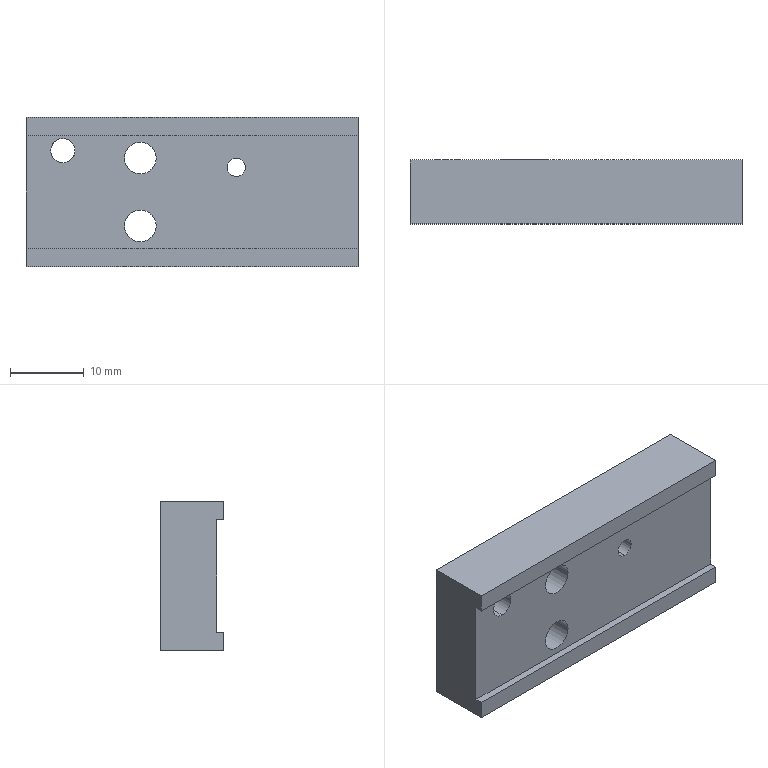Part | NX | 1 solid | 28 faces | box 45 x 8.65 x 20.2 mm | volume 6534 mm3 | plane 12 | cylinder 12 | cone 4 | commonest cylinder face diameters 4.3 x4 8 x4 2.5 x2 3.3 x2
STEP:
#1=CARTESIAN_POINT('',(45.,-1.,0.));
#2=VERTEX_POINT('',#1);
#3=CARTESIAN_POINT('',(45.,7.65,0.));
#4=VERTEX_POINT('',#3);
#5=CARTESIAN_POINT('',(45.,-1.,0.));
#6=DIRECTION('',(0.,1.,0.));
#7=VECTOR('',#6,1000.);
#8=LINE('',#5,#7);
#9=EDGE_CURVE('',#2,#4,#8,.T.);
#10=ORIENTED_EDGE('',*,*,#9,.T.);
#11=CARTESIAN_POINT('',(0.,7.65,0.));
#12=VERTEX_POINT('',#11);
#13=CARTESIAN_POINT('',(0.,7.65,0.));
#14=DIRECTION('',(-1.,0.,0.));
#15=VECTOR('',#14,1000.);
#16=LINE('',#13,#15);
#17=EDGE_CURVE('',#4,#12,#16,.T.);
#18=ORIENTED_EDGE('',*,*,#17,.T.);
#19=CARTESIAN_POINT('',(0.,-1.,0.));
#20=VERTEX_POINT('',#19);
#21=CARTESIAN_POINT('',(0.,7.65,0.));
#22=DIRECTION('',(0.,-1.,0.));
#23=VECTOR('',#22,1000.);
#24=LINE('',#21,#23);
#25=EDGE_CURVE('',#12,#20,#24,.T.);
#26=ORIENTED_EDGE('',*,*,#25,.T.);
#27=CARTESIAN_POINT('',(0.,-1.,0.));
#28=DIRECTION('',(1.,0.,0.));
#29=VECTOR('',#28,1000.);
#30=LINE('',#27,#29);
#31=EDGE_CURVE('',#20,#2,#30,.T.);
#32=ORIENTED_EDGE('',*,*,#31,.T.);
#33=EDGE_LOOP('',(#10,#18,#26,#32));
#34=FACE_BOUND('',#33,.T.);
#35=CARTESIAN_POINT('',(0.,0.,0.));
#36=DIRECTION('',(0.,0.,1.));
#37=DIRECTION('',(1.,0.,0.));
#38=AXIS2_PLACEMENT_3D('',#35,#36,#37);
#39=PLANE('',#38);
#40=ADVANCED_FACE('',(#34),#39,.T.);
#41=CARTESIAN_POINT('',(45.,7.65,-20.2));
#42=VERTEX_POINT('',#41);
#43=CARTESIAN_POINT('',(45.,-1.,-20.2));
#44=VERTEX_POINT('',#43);
#45=CARTESIAN_POINT('',(45.,7.65,-20.2));
#46=DIRECTION('',(0.,-1.,0.));
#47=VECTOR('',#46,1000.);
#48=LINE('',#45,#47);
#49=EDGE_CURVE('',#42,#44,#48,.T.);
#50=ORIENTED_EDGE('',*,*,#49,.F.);
#51=CARTESIAN_POINT('',(45.,7.65,0.));
#52=DIRECTION('',(0.,0.,1.));
#53=VECTOR('',#52,1000.);
#54=LINE('',#51,#53);
#55=EDGE_CURVE('',#42,#4,#54,.T.);
#56=ORIENTED_EDGE('',*,*,#55,.T.);
#57=ORIENTED_EDGE('',*,*,#9,.F.);
#58=CARTESIAN_POINT('',(45.,-1.,-2.5));
#59=VERTEX_POINT('',#58);
#60=CARTESIAN_POINT('',(45.,-1.,0.));
#61=DIRECTION('',(0.,0.,-1.));
#62=VECTOR('',#61,1000.);
#63=LINE('',#60,#62);
#64=EDGE_CURVE('',#2,#59,#63,.T.);
#65=ORIENTED_EDGE('',*,*,#64,.T.);
#66=CARTESIAN_POINT('',(45.,0.,-2.5));
#67=VERTEX_POINT('',#66);
#68=CARTESIAN_POINT('',(45.,-1.,-2.5));
#69=DIRECTION('',(0.,1.,0.));
#70=VECTOR('',#69,1000.);
#71=LINE('',#68,#70);
#72=EDGE_CURVE('',#59,#67,#71,.T.);
#73=ORIENTED_EDGE('',*,*,#72,.T.);
#74=CARTESIAN_POINT('',(45.,0.,-17.7));
#75=VERTEX_POINT('',#74);
#76=CARTESIAN_POINT('',(45.,0.,0.));
#77=DIRECTION('',(0.,0.,-1.));
#78=VECTOR('',#77,1000.);
#79=LINE('',#76,#78);
#80=EDGE_CURVE('',#67,#75,#79,.T.);
#81=ORIENTED_EDGE('',*,*,#80,.T.);
#82=CARTESIAN_POINT('',(45.,-1.,-17.7));
#83=VERTEX_POINT('',#82);
#84=CARTESIAN_POINT('',(45.,-1.,-17.7));
#85=DIRECTION('',(0.,1.,0.));
#86=VECTOR('',#85,1000.);
#87=LINE('',#84,#86);
#88=EDGE_CURVE('',#83,#75,#87,.T.);
#89=ORIENTED_EDGE('',*,*,#88,.F.);
#90=CARTESIAN_POINT('',(45.,-1.,-17.7));
#91=DIRECTION('',(0.,0.,-1.));
#92=VECTOR('',#91,1000.);
#93=LINE('',#90,#92);
#94=EDGE_CURVE('',#83,#44,#93,.T.);
#95=ORIENTED_EDGE('',*,*,#94,.T.);
#96=EDGE_LOOP('',(#50,#56,#57,#65,#73,#81,#89,#95));
#97=FACE_BOUND('',#96,.T.);
#98=CARTESIAN_POINT('',(45.,0.,0.));
#99=DIRECTION('',(1.,0.,0.));
#100=DIRECTION('',(0.,1.,0.));
#101=AXIS2_PLACEMENT_3D('',#98,#99,#100);
#102=PLANE('',#101);
#103=ADVANCED_FACE('',(#97),#102,.T.);
#104=CARTESIAN_POINT('',(0.,-1.,-20.2));
#105=VERTEX_POINT('',#104);
#106=CARTESIAN_POINT('',(0.,7.65,-20.2));
#107=VERTEX_POINT('',#106);
#108=CARTESIAN_POINT('',(0.,-1.,-20.2));
#109=DIRECTION('',(0.,1.,0.));
#110=VECTOR('',#109,1000.);
#111=LINE('',#108,#110);
#112=EDGE_CURVE('',#105,#107,#111,.T.);
#113=ORIENTED_EDGE('',*,*,#112,.T.);
#114=CARTESIAN_POINT('',(0.,7.65,-20.2));
#115=DIRECTION('',(-1.,0.,0.));
#116=VECTOR('',#115,1000.);
#117=LINE('',#114,#116);
#118=EDGE_CURVE('',#42,#107,#117,.T.);
#119=ORIENTED_EDGE('',*,*,#118,.F.);
#120=ORIENTED_EDGE('',*,*,#49,.T.);
#121=CARTESIAN_POINT('',(45.,-1.,-20.2));
#122=DIRECTION('',(-1.,0.,0.));
#123=VECTOR('',#122,1000.);
#124=LINE('',#121,#123);
#125=EDGE_CURVE('',#44,#105,#124,.T.);
#126=ORIENTED_EDGE('',*,*,#125,.T.);
#127=EDGE_LOOP('',(#113,#119,#120,#126));
#128=FACE_BOUND('',#127,.T.);
#129=CARTESIAN_POINT('',(0.,0.,-20.2));
#130=DIRECTION('',(0.,0.,1.));
#131=DIRECTION('',(1.,0.,0.));
#132=AXIS2_PLACEMENT_3D('',#129,#130,#131);
#133=PLANE('',#132);
#134=ADVANCED_FACE('',(#128),#133,.F.);
#135=CARTESIAN_POINT('',(0.,0.,-17.7));
#136=VERTEX_POINT('',#135);
#137=CARTESIAN_POINT('',(0.,0.,-2.5));
#138=VERTEX_POINT('',#137);
#139=CARTESIAN_POINT('',(0.,0.,0.));
#140=DIRECTION('',(0.,0.,1.));
#141=VECTOR('',#140,1000.);
#142=LINE('',#139,#141);
#143=EDGE_CURVE('',#136,#138,#142,.T.);
#144=ORIENTED_EDGE('',*,*,#143,.T.);
#145=CARTESIAN_POINT('',(0.,-1.,-2.5));
#146=VERTEX_POINT('',#145);
#147=CARTESIAN_POINT('',(0.,-1.,-2.5));
#148=DIRECTION('',(0.,1.,0.));
#149=VECTOR('',#148,1000.);
#150=LINE('',#147,#149);
#151=EDGE_CURVE('',#146,#138,#150,.T.);
#152=ORIENTED_EDGE('',*,*,#151,.F.);
#153=CARTESIAN_POINT('',(0.,-1.,-2.5));
#154=DIRECTION('',(0.,0.,1.));
#155=VECTOR('',#154,1000.);
#156=LINE('',#153,#155);
#157=EDGE_CURVE('',#146,#20,#156,.T.);
#158=ORIENTED_EDGE('',*,*,#157,.T.);
#159=ORIENTED_EDGE('',*,*,#25,.F.);
#160=CARTESIAN_POINT('',(0.,7.65,0.));
#161=DIRECTION('',(0.,0.,-1.));
#162=VECTOR('',#161,1000.);
#163=LINE('',#160,#162);
#164=EDGE_CURVE('',#12,#107,#163,.T.);
#165=ORIENTED_EDGE('',*,*,#164,.T.);
#166=ORIENTED_EDGE('',*,*,#112,.F.);
#167=CARTESIAN_POINT('',(0.,-1.,-17.7));
#168=VERTEX_POINT('',#167);
#169=CARTESIAN_POINT('',(0.,-1.,-20.2));
#170=DIRECTION('',(0.,0.,1.));
#171=VECTOR('',#170,1000.);
#172=LINE('',#169,#171);
#173=EDGE_CURVE('',#105,#168,#172,.T.);
#174=ORIENTED_EDGE('',*,*,#173,.T.);
#175=CARTESIAN_POINT('',(0.,-1.,-17.7));
#176=DIRECTION('',(0.,1.,0.));
#177=VECTOR('',#176,1000.);
#178=LINE('',#175,#177);
#179=EDGE_CURVE('',#168,#136,#178,.T.);
#180=ORIENTED_EDGE('',*,*,#179,.T.);
#181=EDGE_LOOP('',(#144,#152,#158,#159,#165,#166,#174,#180));
#182=FACE_BOUND('',#181,.T.);
#183=CARTESIAN_POINT('',(0.,7.65,0.));
#184=DIRECTION('',(-1.,0.,0.));
#185=DIRECTION('',(0.,0.,1.));
#186=AXIS2_PLACEMENT_3D('',#183,#184,#185);
#187=PLANE('',#186);
#188=ADVANCED_FACE('',(#182),#187,.T.);
#189=CARTESIAN_POINT('',(0.,0.,-2.5));
#190=DIRECTION('',(-1.,0.,0.));
#191=VECTOR('',#190,1000.);
#192=LINE('',#189,#191);
#193=EDGE_CURVE('',#67,#138,#192,.T.);
#194=ORIENTED_EDGE('',*,*,#193,.T.);
#195=ORIENTED_EDGE('',*,*,#143,.F.);
#196=CARTESIAN_POINT('',(0.,0.,-17.7));
#197=DIRECTION('',(1.,0.,0.));
#198=VECTOR('',#197,1000.);
#199=LINE('',#196,#198);
#200=EDGE_CURVE('',#136,#75,#199,.T.);
#201=ORIENTED_EDGE('',*,*,#200,.T.);
#202=ORIENTED_EDGE('',*,*,#80,.F.);
#203=EDGE_LOOP('',(#194,#195,#201,#202));
#204=FACE_BOUND('',#203,.T.);
#205=CARTESIAN_POINT('',(13.35,0.,-14.7));
#206=VERTEX_POINT('',#205);
#207=CARTESIAN_POINT('',(17.65,0.,-14.7));
#208=VERTEX_POINT('',#207);
#209=CARTESIAN_POINT('',(15.5,0.,-14.7));
#210=DIRECTION('',(0.,1.,0.));
#211=DIRECTION('',(1.,0.,0.));
#212=AXIS2_PLACEMENT_3D('',#209,#210,#211);
#213=CIRCLE('',#212,2.15);
#214=EDGE_CURVE('',#206,#208,#213,.T.);
#215=ORIENTED_EDGE('',*,*,#214,.T.);
#216=CARTESIAN_POINT('',(15.5,0.,-14.7));
#217=DIRECTION('',(0.,1.,0.));
#218=DIRECTION('',(1.,0.,0.));
#219=AXIS2_PLACEMENT_3D('',#216,#217,#218);
#220=CIRCLE('',#219,2.15);
#221=EDGE_CURVE('',#208,#206,#220,.T.);
#222=ORIENTED_EDGE('',*,*,#221,.T.);
#223=EDGE_LOOP('',(#215,#222));
#224=FACE_BOUND('',#223,.T.);
#225=CARTESIAN_POINT('',(13.35,0.,-5.5));
#226=VERTEX_POINT('',#225);
#227=CARTESIAN_POINT('',(17.65,0.,-5.5));
#228=VERTEX_POINT('',#227);
#229=CARTESIAN_POINT('',(15.5,0.,-5.5));
#230=DIRECTION('',(0.,1.,0.));
#231=DIRECTION('',(1.,0.,0.));
#232=AXIS2_PLACEMENT_3D('',#229,#230,#231);
#233=CIRCLE('',#232,2.15);
#234=EDGE_CURVE('',#226,#228,#233,.T.);
#235=ORIENTED_EDGE('',*,*,#234,.T.);
#236=CARTESIAN_POINT('',(15.5,0.,-5.5));
#237=DIRECTION('',(0.,1.,0.));
#238=DIRECTION('',(1.,0.,0.));
#239=AXIS2_PLACEMENT_3D('',#236,#237,#238);
#240=CIRCLE('',#239,2.15);
#241=EDGE_CURVE('',#228,#226,#240,.T.);
#242=ORIENTED_EDGE('',*,*,#241,.T.);
#243=EDGE_LOOP('',(#235,#242));
#244=FACE_BOUND('',#243,.T.);
#245=CARTESIAN_POINT('',(5.,0.,-2.85));
#246=VERTEX_POINT('',#245);
#247=CARTESIAN_POINT('',(5.,0.,-6.15));
#248=VERTEX_POINT('',#247);
#249=CARTESIAN_POINT('',(5.,0.,-4.5));
#250=DIRECTION('',(0.,1.,0.));
#251=DIRECTION('',(0.,0.,-1.));
#252=AXIS2_PLACEMENT_3D('',#249,#250,#251);
#253=CIRCLE('',#252,1.65);
#254=EDGE_CURVE('',#246,#248,#253,.T.);
#255=ORIENTED_EDGE('',*,*,#254,.T.);
#256=CARTESIAN_POINT('',(5.,0.,-4.5));
#257=DIRECTION('',(0.,1.,0.));
#258=DIRECTION('',(0.,0.,-1.));
#259=AXIS2_PLACEMENT_3D('',#256,#257,#258);
#260=CIRCLE('',#259,1.65);
#261=EDGE_CURVE('',#248,#246,#260,.T.);
#262=ORIENTED_EDGE('',*,*,#261,.T.);
#263=EDGE_LOOP('',(#255,#262));
#264=FACE_BOUND('',#263,.T.);
#265=CARTESIAN_POINT('',(28.5,0.,-5.5));
#266=VERTEX_POINT('',#265);
#267=CARTESIAN_POINT('',(28.5,0.,-8.));
#268=VERTEX_POINT('',#267);
#269=CARTESIAN_POINT('',(28.5,0.,-6.75));
#270=DIRECTION('',(0.,1.,0.));
#271=DIRECTION('',(0.,0.,-1.));
#272=AXIS2_PLACEMENT_3D('',#269,#270,#271);
#273=CIRCLE('',#272,1.25);
#274=EDGE_CURVE('',#266,#268,#273,.T.);
#275=ORIENTED_EDGE('',*,*,#274,.T.);
#276=CARTESIAN_POINT('',(28.5,0.,-6.75));
#277=DIRECTION('',(0.,1.,0.));
#278=DIRECTION('',(0.,0.,-1.));
#279=AXIS2_PLACEMENT_3D('',#276,#277,#278);
#280=CIRCLE('',#279,1.25);
#281=EDGE_CURVE('',#268,#266,#280,.T.);
#282=ORIENTED_EDGE('',*,*,#281,.T.);
#283=EDGE_LOOP('',(#275,#282));
#284=FACE_BOUND('',#283,.T.);
#285=CARTESIAN_POINT('',(0.,0.,0.));
#286=DIRECTION('',(0.,-1.,0.));
#287=DIRECTION('',(0.,0.,-1.));
#288=AXIS2_PLACEMENT_3D('',#285,#286,#287);
#289=PLANE('',#288);
#290=ADVANCED_FACE('',(#204,#224,#244,#264,#284),#289,.T.);
#291=ORIENTED_EDGE('',*,*,#193,.F.);
#292=ORIENTED_EDGE('',*,*,#72,.F.);
#293=CARTESIAN_POINT('',(45.,-1.,-2.5));
#294=DIRECTION('',(-1.,0.,0.));
#295=VECTOR('',#294,1000.);
#296=LINE('',#293,#295);
#297=EDGE_CURVE('',#59,#146,#296,.T.);
#298=ORIENTED_EDGE('',*,*,#297,.T.);
#299=ORIENTED_EDGE('',*,*,#151,.T.);
#300=EDGE_LOOP('',(#291,#292,#298,#299));
#301=FACE_BOUND('',#300,.T.);
#302=CARTESIAN_POINT('',(0.,0.,-2.5));
#303=DIRECTION('',(0.,0.,-1.));
#304=DIRECTION('',(0.,-1.,0.));
#305=AXIS2_PLACEMENT_3D('',#302,#303,#304);
#306=PLANE('',#305);
#307=ADVANCED_FACE('',(#301),#306,.T.);
#308=ORIENTED_EDGE('',*,*,#157,.F.);
#309=ORIENTED_EDGE('',*,*,#297,.F.);
#310=ORIENTED_EDGE('',*,*,#64,.F.);
#311=ORIENTED_EDGE('',*,*,#31,.F.);
#312=EDGE_LOOP('',(#308,#309,#310,#311));
#313=FACE_BOUND('',#312,.T.);
#314=CARTESIAN_POINT('',(0.,-1.,0.));
#315=DIRECTION('',(0.,-1.,0.));
#316=DIRECTION('',(0.,0.,-1.));
#317=AXIS2_PLACEMENT_3D('',#314,#315,#316);
#318=PLANE('',#317);
#319=ADVANCED_FACE('',(#313),#318,.T.);
#320=ORIENTED_EDGE('',*,*,#200,.F.);
#321=ORIENTED_EDGE('',*,*,#179,.F.);
#322=CARTESIAN_POINT('',(0.,-1.,-17.7));
#323=DIRECTION('',(1.,0.,0.));
#324=VECTOR('',#323,1000.);
#325=LINE('',#322,#324);
#326=EDGE_CURVE('',#168,#83,#325,.T.);
#327=ORIENTED_EDGE('',*,*,#326,.T.);
#328=ORIENTED_EDGE('',*,*,#88,.T.);
#329=EDGE_LOOP('',(#320,#321,#327,#328));
#330=FACE_BOUND('',#329,.T.);
#331=CARTESIAN_POINT('',(45.,0.,-17.7));
#332=DIRECTION('',(0.,0.,1.));
#333=DIRECTION('',(1.,0.,0.));
#334=AXIS2_PLACEMENT_3D('',#331,#332,#333);
#335=PLANE('',#334);
#336=ADVANCED_FACE('',(#330),#335,.T.);
#337=ORIENTED_EDGE('',*,*,#125,.F.);
#338=ORIENTED_EDGE('',*,*,#94,.F.);
#339=ORIENTED_EDGE('',*,*,#326,.F.);
#340=ORIENTED_EDGE('',*,*,#173,.F.);
#341=EDGE_LOOP('',(#337,#338,#339,#340));
#342=FACE_BOUND('',#341,.T.);
#343=CARTESIAN_POINT('',(0.,-1.,0.));
#344=DIRECTION('',(0.,-1.,0.));
#345=DIRECTION('',(0.,0.,-1.));
#346=AXIS2_PLACEMENT_3D('',#343,#344,#345);
#347=PLANE('',#346);
#348=ADVANCED_FACE('',(#342),#347,.T.);
#349=CARTESIAN_POINT('',(17.65,3.25,-14.7));
#350=VERTEX_POINT('',#349);
#351=CARTESIAN_POINT('',(13.35,3.25,-14.7));
#352=VERTEX_POINT('',#351);
#353=CARTESIAN_POINT('',(15.5,3.25,-14.7));
#354=DIRECTION('',(0.,1.,0.));
#355=DIRECTION('',(-1.,0.,0.));
#356=AXIS2_PLACEMENT_3D('',#353,#354,#355);
#357=CIRCLE('',#356,2.15);
#358=EDGE_CURVE('',#350,#352,#357,.T.);
#359=ORIENTED_EDGE('',*,*,#358,.T.);
#360=CARTESIAN_POINT('',(13.35,-2.341,-14.7));
#361=DIRECTION('',(0.,1.,0.));
#362=VECTOR('',#361,1000.);
#363=LINE('',#360,#362);
#364=EDGE_CURVE('',#352,#206,#363,.F.);
#365=ORIENTED_EDGE('',*,*,#364,.T.);
#366=ORIENTED_EDGE('',*,*,#221,.F.);
#367=CARTESIAN_POINT('',(17.65,-2.341,-14.7));
#368=DIRECTION('',(0.,1.,0.));
#369=VECTOR('',#368,1000.);
#370=LINE('',#367,#369);
#371=EDGE_CURVE('',#350,#208,#370,.F.);
#372=ORIENTED_EDGE('',*,*,#371,.F.);
#373=EDGE_LOOP('',(#359,#365,#366,#372));
#374=FACE_BOUND('',#373,.T.);
#375=CARTESIAN_POINT('',(15.5,-2.341,-14.7));
#376=DIRECTION('',(0.,1.,0.));
#377=DIRECTION('',(1.,0.,0.));
#378=AXIS2_PLACEMENT_3D('',#375,#376,#377);
#379=CYLINDRICAL_SURFACE('',#378,2.15);
#380=ADVANCED_FACE('',(#374),#379,.F.);
#381=ORIENTED_EDGE('',*,*,#234,.F.);
#382=CARTESIAN_POINT('',(13.35,3.15,-5.5));
#383=VERTEX_POINT('',#382);
#384=CARTESIAN_POINT('',(13.35,-2.341,-5.5));
#385=DIRECTION('',(0.,1.,0.));
#386=VECTOR('',#385,1000.);
#387=LINE('',#384,#386);
#388=EDGE_CURVE('',#226,#383,#387,.T.);
#389=ORIENTED_EDGE('',*,*,#388,.T.);
#390=CARTESIAN_POINT('',(17.65,3.15,-5.5));
#391=VERTEX_POINT('',#390);
#392=CARTESIAN_POINT('',(15.5,3.15,-5.5));
#393=DIRECTION('',(0.,1.,0.));
#394=DIRECTION('',(1.,0.,0.));
#395=AXIS2_PLACEMENT_3D('',#392,#393,#394);
#396=CIRCLE('',#395,2.15);
#397=EDGE_CURVE('',#383,#391,#396,.T.);
#398=ORIENTED_EDGE('',*,*,#397,.T.);
#399=CARTESIAN_POINT('',(17.65,-2.341,-5.5));
#400=DIRECTION('',(0.,1.,0.));
#401=VECTOR('',#400,1000.);
#402=LINE('',#399,#401);
#403=EDGE_CURVE('',#228,#391,#402,.T.);
#404=ORIENTED_EDGE('',*,*,#403,.F.);
#405=EDGE_LOOP('',(#381,#389,#398,#404));
#406=FACE_BOUND('',#405,.T.);
#407=CARTESIAN_POINT('',(15.5,-2.341,-5.5));
#408=DIRECTION('',(0.,1.,0.));
#409=DIRECTION('',(1.,0.,0.));
#410=AXIS2_PLACEMENT_3D('',#407,#408,#409);
#411=CYLINDRICAL_SURFACE('',#410,2.15);
#412=ADVANCED_FACE('',(#406),#411,.F.);
#413=CARTESIAN_POINT('',(19.5,3.25,-14.7));
#414=VERTEX_POINT('',#413);
#415=CARTESIAN_POINT('',(11.5,3.25,-14.7));
#416=VERTEX_POINT('',#415);
#417=CARTESIAN_POINT('',(15.5,3.25,-14.7));
#418=DIRECTION('',(0.,-1.,0.));
#419=DIRECTION('',(1.,0.,0.));
#420=AXIS2_PLACEMENT_3D('',#417,#418,#419);
#421=CIRCLE('',#420,4.);
#422=EDGE_CURVE('',#414,#416,#421,.T.);
#423=ORIENTED_EDGE('',*,*,#422,.F.);
#424=CARTESIAN_POINT('',(15.5,3.25,-14.7));
#425=DIRECTION('',(0.,-1.,0.));
#426=DIRECTION('',(1.,0.,0.));
#427=AXIS2_PLACEMENT_3D('',#424,#425,#426);
#428=CIRCLE('',#427,4.);
#429=EDGE_CURVE('',#416,#414,#428,.T.);
#430=ORIENTED_EDGE('',*,*,#429,.F.);
#431=EDGE_LOOP('',(#423,#430));
#432=FACE_BOUND('',#431,.T.);
#433=ORIENTED_EDGE('',*,*,#358,.F.);
#434=CARTESIAN_POINT('',(15.5,3.25,-14.7));
#435=DIRECTION('',(0.,1.,0.));
#436=DIRECTION('',(-1.,0.,0.));
#437=AXIS2_PLACEMENT_3D('',#434,#435,#436);
#438=CIRCLE('',#437,2.15);
#439=EDGE_CURVE('',#352,#350,#438,.T.);
#440=ORIENTED_EDGE('',*,*,#439,.F.);
#441=EDGE_LOOP('',(#433,#440));
#442=FACE_BOUND('',#441,.T.);
#443=CARTESIAN_POINT('',(15.5,3.25,-14.7));
#444=DIRECTION('',(0.,1.,0.));
#445=DIRECTION('',(1.,0.,0.));
#446=AXIS2_PLACEMENT_3D('',#443,#444,#445);
#447=PLANE('',#446);
#448=ADVANCED_FACE('',(#432,#442),#447,.T.);
#449=CARTESIAN_POINT('',(19.5,7.65,-14.7));
#450=VERTEX_POINT('',#449);
#451=CARTESIAN_POINT('',(11.5,7.65,-14.7));
#452=VERTEX_POINT('',#451);
#453=CARTESIAN_POINT('',(15.5,7.65,-14.7));
#454=DIRECTION('',(0.,1.,0.));
#455=DIRECTION('',(1.,0.,0.));
#456=AXIS2_PLACEMENT_3D('',#453,#454,#455);
#457=CIRCLE('',#456,4.);
#458=EDGE_CURVE('',#450,#452,#457,.T.);
#459=ORIENTED_EDGE('',*,*,#458,.T.);
#460=CARTESIAN_POINT('',(11.5,-2.341,-14.7));
#461=DIRECTION('',(0.,1.,0.));
#462=VECTOR('',#461,1000.);
#463=LINE('',#460,#462);
#464=EDGE_CURVE('',#452,#416,#463,.F.);
#465=ORIENTED_EDGE('',*,*,#464,.T.);
#466=ORIENTED_EDGE('',*,*,#429,.T.);
#467=CARTESIAN_POINT('',(19.5,-2.341,-14.7));
#468=DIRECTION('',(0.,1.,0.));
#469=VECTOR('',#468,1000.);
#470=LINE('',#467,#469);
#471=EDGE_CURVE('',#450,#414,#470,.F.);
#472=ORIENTED_EDGE('',*,*,#471,.F.);
#473=EDGE_LOOP('',(#459,#465,#466,#472));
#474=FACE_BOUND('',#473,.T.);
#475=CARTESIAN_POINT('',(15.5,-2.341,-14.7));
#476=DIRECTION('',(0.,1.,0.));
#477=DIRECTION('',(1.,0.,0.));
#478=AXIS2_PLACEMENT_3D('',#475,#476,#477);
#479=CYLINDRICAL_SURFACE('',#478,4.);
#480=ADVANCED_FACE('',(#474),#479,.F.);
#481=ORIENTED_EDGE('',*,*,#17,.F.);
#482=ORIENTED_EDGE('',*,*,#55,.F.);
#483=ORIENTED_EDGE('',*,*,#118,.T.);
#484=ORIENTED_EDGE('',*,*,#164,.F.);
#485=EDGE_LOOP('',(#481,#482,#483,#484));
#486=FACE_BOUND('',#485,.T.);
#487=ORIENTED_EDGE('',*,*,#458,.F.);
#488=CARTESIAN_POINT('',(15.5,7.65,-14.7));
#489=DIRECTION('',(0.,1.,0.));
#490=DIRECTION('',(1.,0.,0.));
#491=AXIS2_PLACEMENT_3D('',#488,#489,#490);
#492=CIRCLE('',#491,4.);
#493=EDGE_CURVE('',#452,#450,#492,.T.);
#494=ORIENTED_EDGE('',*,*,#493,.F.);
#495=EDGE_LOOP('',(#487,#494));
#496=FACE_BOUND('',#495,.T.);
#497=CARTESIAN_POINT('',(30.2,7.65,-6.75));
#498=VERTEX_POINT('',#497);
#499=CARTESIAN_POINT('',(26.8,7.65,-6.75));
#500=VERTEX_POINT('',#499);
#501=CARTESIAN_POINT('',(28.5,7.65,-6.75));
#502=DIRECTION('',(0.,1.,0.));
#503=DIRECTION('',(1.,0.,0.));
#504=AXIS2_PLACEMENT_3D('',#501,#502,#503);
#505=CIRCLE('',#504,1.7);
#506=EDGE_CURVE('',#498,#500,#505,.T.);
#507=ORIENTED_EDGE('',*,*,#506,.F.);
#508=CARTESIAN_POINT('',(28.5,7.65,-6.75));
#509=DIRECTION('',(0.,1.,0.));
#510=DIRECTION('',(1.,0.,0.));
#511=AXIS2_PLACEMENT_3D('',#508,#509,#510);
#512=CIRCLE('',#511,1.7);
#513=EDGE_CURVE('',#500,#498,#512,.T.);
#514=ORIENTED_EDGE('',*,*,#513,.F.);
#515=EDGE_LOOP('',(#507,#514));
#516=FACE_BOUND('',#515,.T.);
#517=CARTESIAN_POINT('',(11.5,7.65,-5.5));
#518=VERTEX_POINT('',#517);
#519=CARTESIAN_POINT('',(19.5,7.65,-5.5));
#520=VERTEX_POINT('',#519);
#521=CARTESIAN_POINT('',(15.5,7.65,-5.5));
#522=DIRECTION('',(0.,1.,0.));
#523=DIRECTION('',(1.,0.,0.));
#524=AXIS2_PLACEMENT_3D('',#521,#522,#523);
#525=CIRCLE('',#524,4.);
#526=EDGE_CURVE('',#518,#520,#525,.T.);
#527=ORIENTED_EDGE('',*,*,#526,.F.);
#528=CARTESIAN_POINT('',(15.5,7.65,-5.5));
#529=DIRECTION('',(0.,1.,0.));
#530=DIRECTION('',(1.,0.,0.));
#531=AXIS2_PLACEMENT_3D('',#528,#529,#530);
#532=CIRCLE('',#531,4.);
#533=EDGE_CURVE('',#520,#518,#532,.T.);
#534=ORIENTED_EDGE('',*,*,#533,.F.);
#535=EDGE_LOOP('',(#527,#534));
#536=FACE_BOUND('',#535,.T.);
#537=CARTESIAN_POINT('',(2.685,7.65,-4.5));
#538=VERTEX_POINT('',#537);
#539=CARTESIAN_POINT('',(7.315,7.65,-4.5));
#540=VERTEX_POINT('',#539);
#541=CARTESIAN_POINT('',(5.,7.65,-4.5));
#542=DIRECTION('',(0.,1.,0.));
#543=DIRECTION('',(1.,0.,0.));
#544=AXIS2_PLACEMENT_3D('',#541,#542,#543);
#545=CIRCLE('',#544,2.315);
#546=EDGE_CURVE('',#538,#540,#545,.T.);
#547=ORIENTED_EDGE('',*,*,#546,.F.);
#548=CARTESIAN_POINT('',(5.,7.65,-4.5));
#549=DIRECTION('',(0.,1.,0.));
#550=DIRECTION('',(1.,0.,0.));
#551=AXIS2_PLACEMENT_3D('',#548,#549,#550);
#552=CIRCLE('',#551,2.315);
#553=EDGE_CURVE('',#540,#538,#552,.T.);
#554=ORIENTED_EDGE('',*,*,#553,.F.);
#555=EDGE_LOOP('',(#547,#554));
#556=FACE_BOUND('',#555,.T.);
#557=CARTESIAN_POINT('',(45.,7.65,0.));
#558=DIRECTION('',(0.,1.,0.));
#559=DIRECTION('',(1.,0.,0.));
#560=AXIS2_PLACEMENT_3D('',#557,#558,#559);
#561=PLANE('',#560);
#562=ADVANCED_FACE('',(#486,#496,#516,#536,#556),#561,.T.);
#563=CARTESIAN_POINT('',(11.5,3.15,-5.5));
#564=VERTEX_POINT('',#563);
#565=CARTESIAN_POINT('',(19.5,3.15,-5.5));
#566=VERTEX_POINT('',#565);
#567=CARTESIAN_POINT('',(15.5,3.15,-5.5));
#568=DIRECTION('',(0.,-1.,0.));
#569=DIRECTION('',(1.,0.,0.));
#570=AXIS2_PLACEMENT_3D('',#567,#568,#569);
#571=CIRCLE('',#570,4.);
#572=EDGE_CURVE('',#564,#566,#571,.T.);
#573=ORIENTED_EDGE('',*,*,#572,.F.);
#574=CARTESIAN_POINT('',(15.5,3.15,-5.5));
#575=DIRECTION('',(0.,-1.,0.));
#576=DIRECTION('',(1.,0.,0.));
#577=AXIS2_PLACEMENT_3D('',#574,#575,#576);
#578=CIRCLE('',#577,4.);
#579=EDGE_CURVE('',#566,#564,#578,.T.);
#580=ORIENTED_EDGE('',*,*,#579,.F.);
#581=EDGE_LOOP('',(#573,#580));
#582=FACE_BOUND('',#581,.T.);
#583=ORIENTED_EDGE('',*,*,#397,.F.);
#584=CARTESIAN_POINT('',(15.5,3.15,-5.5));
#585=DIRECTION('',(0.,1.,0.));
#586=DIRECTION('',(1.,0.,0.));
#587=AXIS2_PLACEMENT_3D('',#584,#585,#586);
#588=CIRCLE('',#587,2.15);
#589=EDGE_CURVE('',#391,#383,#588,.T.);
#590=ORIENTED_EDGE('',*,*,#589,.F.);
#591=EDGE_LOOP('',(#583,#590));
#592=FACE_BOUND('',#591,.T.);
#593=CARTESIAN_POINT('',(15.5,3.15,-5.5));
#594=DIRECTION('',(0.,1.,0.));
#595=DIRECTION('',(1.,0.,0.));
#596=AXIS2_PLACEMENT_3D('',#593,#594,#595);
#597=PLANE('',#596);
#598=ADVANCED_FACE('',(#582,#592),#597,.T.);
#599=ORIENTED_EDGE('',*,*,#526,.T.);
#600=CARTESIAN_POINT('',(19.5,-2.341,-5.5));
#601=DIRECTION('',(0.,1.,0.));
#602=VECTOR('',#601,1000.);
#603=LINE('',#600,#602);
#604=EDGE_CURVE('',#566,#520,#603,.T.);
#605=ORIENTED_EDGE('',*,*,#604,.F.);
#606=ORIENTED_EDGE('',*,*,#579,.T.);
#607=CARTESIAN_POINT('',(11.5,-2.341,-5.5));
#608=DIRECTION('',(0.,1.,0.));
#609=VECTOR('',#608,1000.);
#610=LINE('',#607,#609);
#611=EDGE_CURVE('',#564,#518,#610,.T.);
#612=ORIENTED_EDGE('',*,*,#611,.T.);
#613=EDGE_LOOP('',(#599,#605,#606,#612));
#614=FACE_BOUND('',#613,.T.);
#615=CARTESIAN_POINT('',(15.5,-2.341,-5.5));
#616=DIRECTION('',(0.,1.,0.));
#617=DIRECTION('',(1.,0.,0.));
#618=AXIS2_PLACEMENT_3D('',#615,#616,#617);
#619=CYLINDRICAL_SURFACE('',#618,4.);
#620=ADVANCED_FACE('',(#614),#619,.F.);
#621=ORIENTED_EDGE('',*,*,#254,.F.);
#622=CARTESIAN_POINT('',(5.,7.266,-2.85));
#623=VERTEX_POINT('',#622);
#624=CARTESIAN_POINT('',(5.,3.825,-2.85));
#625=DIRECTION('',(0.,1.,0.));
#626=VECTOR('',#625,1000.);
#627=LINE('',#624,#626);
#628=EDGE_CURVE('',#246,#623,#627,.T.);
#629=ORIENTED_EDGE('',*,*,#628,.T.);
#630=CARTESIAN_POINT('',(6.65,7.266,-4.5));
#631=VERTEX_POINT('',#630);
#632=CARTESIAN_POINT('',(5.,7.266,-4.5));
#633=DIRECTION('',(0.,1.,0.));
#634=DIRECTION('',(1.,0.,0.));
#635=AXIS2_PLACEMENT_3D('',#632,#633,#634);
#636=CIRCLE('',#635,1.65);
#637=EDGE_CURVE('',#623,#631,#636,.T.);
#638=ORIENTED_EDGE('',*,*,#637,.T.);
#639=CARTESIAN_POINT('',(5.,7.266,-6.15));
#640=VERTEX_POINT('',#639);
#641=CARTESIAN_POINT('',(5.,7.266,-4.5));
#642=DIRECTION('',(0.,1.,0.));
#643=DIRECTION('',(1.,0.,0.));
#644=AXIS2_PLACEMENT_3D('',#641,#642,#643);
#645=CIRCLE('',#644,1.65);
#646=EDGE_CURVE('',#631,#640,#645,.T.);
#647=ORIENTED_EDGE('',*,*,#646,.T.);
#648=CARTESIAN_POINT('',(5.,3.825,-6.15));
#649=DIRECTION('',(0.,1.,0.));
#650=VECTOR('',#649,1000.);
#651=LINE('',#648,#650);
#652=EDGE_CURVE('',#248,#640,#651,.T.);
#653=ORIENTED_EDGE('',*,*,#652,.F.);
#654=EDGE_LOOP('',(#621,#629,#638,#647,#653));
#655=FACE_BOUND('',#654,.T.);
#656=CARTESIAN_POINT('',(5.,3.825,-4.5));
#657=DIRECTION('',(0.,1.,0.));
#658=DIRECTION('',(0.,0.,-1.));
#659=AXIS2_PLACEMENT_3D('',#656,#657,#658);
#660=CYLINDRICAL_SURFACE('',#659,1.65);
#661=ADVANCED_FACE('',(#655),#660,.F.);
#662=ORIENTED_EDGE('',*,*,#546,.T.);
#663=CARTESIAN_POINT('',(6.65,7.266,-4.5));
#664=DIRECTION('',(0.866,0.5,0.));
#665=VECTOR('',#664,1000.);
#666=LINE('',#663,#665);
#667=EDGE_CURVE('',#631,#540,#666,.T.);
#668=ORIENTED_EDGE('',*,*,#667,.F.);
#669=ORIENTED_EDGE('',*,*,#637,.F.);
#670=CARTESIAN_POINT('',(3.35,7.266,-4.5));
#671=VERTEX_POINT('',#670);
#672=CARTESIAN_POINT('',(5.,7.266,-4.5));
#673=DIRECTION('',(0.,1.,0.));
#674=DIRECTION('',(1.,0.,0.));
#675=AXIS2_PLACEMENT_3D('',#672,#673,#674);
#676=CIRCLE('',#675,1.65);
#677=EDGE_CURVE('',#671,#623,#676,.T.);
#678=ORIENTED_EDGE('',*,*,#677,.F.);
#679=CARTESIAN_POINT('',(3.35,7.266,-4.5));
#680=DIRECTION('',(-0.866,0.5,0.));
#681=VECTOR('',#680,1000.);
#682=LINE('',#679,#681);
#683=EDGE_CURVE('',#671,#538,#682,.T.);
#684=ORIENTED_EDGE('',*,*,#683,.T.);
#685=EDGE_LOOP('',(#662,#668,#669,#678,#684));
#686=FACE_BOUND('',#685,.T.);
#687=CARTESIAN_POINT('',(5.,7.266,-4.5));
#688=DIRECTION('',(0.,1.,0.));
#689=DIRECTION('',(1.,0.,0.));
#690=AXIS2_PLACEMENT_3D('',#687,#688,#689);
#691=CONICAL_SURFACE('',#690,1.65,1.047);
#692=ADVANCED_FACE('',(#686),#691,.F.);
#693=ORIENTED_EDGE('',*,*,#274,.F.);
#694=CARTESIAN_POINT('',(28.5,7.39,-5.5));
#695=VERTEX_POINT('',#694);
#696=CARTESIAN_POINT('',(28.5,3.825,-5.5));
#697=DIRECTION('',(0.,1.,0.));
#698=VECTOR('',#697,1000.);
#699=LINE('',#696,#698);
#700=EDGE_CURVE('',#266,#695,#699,.T.);
#701=ORIENTED_EDGE('',*,*,#700,.T.);
#702=CARTESIAN_POINT('',(29.75,7.39,-6.75));
#703=VERTEX_POINT('',#702);
#704=CARTESIAN_POINT('',(28.5,7.39,-6.75));
#705=DIRECTION('',(0.,1.,0.));
#706=DIRECTION('',(1.,0.,0.));
#707=AXIS2_PLACEMENT_3D('',#704,#705,#706);
#708=CIRCLE('',#707,1.25);
#709=EDGE_CURVE('',#695,#703,#708,.T.);
#710=ORIENTED_EDGE('',*,*,#709,.T.);
#711=CARTESIAN_POINT('',(28.5,7.39,-8.));
#712=VERTEX_POINT('',#711);
#713=CARTESIAN_POINT('',(28.5,7.39,-6.75));
#714=DIRECTION('',(0.,1.,0.));
#715=DIRECTION('',(1.,0.,0.));
#716=AXIS2_PLACEMENT_3D('',#713,#714,#715);
#717=CIRCLE('',#716,1.25);
#718=EDGE_CURVE('',#703,#712,#717,.T.);
#719=ORIENTED_EDGE('',*,*,#718,.T.);
#720=CARTESIAN_POINT('',(28.5,3.825,-8.));
#721=DIRECTION('',(0.,1.,0.));
#722=VECTOR('',#721,1000.);
#723=LINE('',#720,#722);
#724=EDGE_CURVE('',#268,#712,#723,.T.);
#725=ORIENTED_EDGE('',*,*,#724,.F.);
#726=EDGE_LOOP('',(#693,#701,#710,#719,#725));
#727=FACE_BOUND('',#726,.T.);
#728=CARTESIAN_POINT('',(28.5,3.825,-6.75));
#729=DIRECTION('',(0.,1.,0.));
#730=DIRECTION('',(0.,0.,-1.));
#731=AXIS2_PLACEMENT_3D('',#728,#729,#730);
#732=CYLINDRICAL_SURFACE('',#731,1.25);
#733=ADVANCED_FACE('',(#727),#732,.F.);
#734=ORIENTED_EDGE('',*,*,#506,.T.);
#735=CARTESIAN_POINT('',(27.25,7.39,-6.75));
#736=VERTEX_POINT('',#735);
#737=CARTESIAN_POINT('',(27.25,7.39,-6.75));
#738=DIRECTION('',(-0.866,0.5,0.));
#739=VECTOR('',#738,1000.);
#740=LINE('',#737,#739);
#741=EDGE_CURVE('',#500,#736,#740,.F.);
#742=ORIENTED_EDGE('',*,*,#741,.T.);
#743=CARTESIAN_POINT('',(28.5,7.39,-6.75));
#744=DIRECTION('',(0.,1.,0.));
#745=DIRECTION('',(1.,0.,0.));
#746=AXIS2_PLACEMENT_3D('',#743,#744,#745);
#747=CIRCLE('',#746,1.25);
#748=EDGE_CURVE('',#712,#736,#747,.T.);
#749=ORIENTED_EDGE('',*,*,#748,.F.);
#750=ORIENTED_EDGE('',*,*,#718,.F.);
#751=CARTESIAN_POINT('',(29.75,7.39,-6.75));
#752=DIRECTION('',(0.866,0.5,0.));
#753=VECTOR('',#752,1000.);
#754=LINE('',#751,#753);
#755=EDGE_CURVE('',#498,#703,#754,.F.);
#756=ORIENTED_EDGE('',*,*,#755,.F.);
#757=EDGE_LOOP('',(#734,#742,#749,#750,#756));
#758=FACE_BOUND('',#757,.T.);
#759=CARTESIAN_POINT('',(28.5,7.39,-6.75));
#760=DIRECTION('',(0.,1.,0.));
#761=DIRECTION('',(1.,0.,0.));
#762=AXIS2_PLACEMENT_3D('',#759,#760,#761);
#763=CONICAL_SURFACE('',#762,1.25,1.047);
#764=ADVANCED_FACE('',(#758),#763,.F.);
#765=ORIENTED_EDGE('',*,*,#403,.T.);
#766=ORIENTED_EDGE('',*,*,#589,.T.);
#767=ORIENTED_EDGE('',*,*,#388,.F.);
#768=ORIENTED_EDGE('',*,*,#241,.F.);
#769=EDGE_LOOP('',(#765,#766,#767,#768));
#770=FACE_BOUND('',#769,.T.);
#771=CARTESIAN_POINT('',(15.5,-2.341,-5.5));
#772=DIRECTION('',(0.,1.,0.));
#773=DIRECTION('',(1.,0.,0.));
#774=AXIS2_PLACEMENT_3D('',#771,#772,#773);
#775=CYLINDRICAL_SURFACE('',#774,2.15);
#776=ADVANCED_FACE('',(#770),#775,.F.);
#777=CARTESIAN_POINT('',(28.5,7.39,-6.75));
#778=DIRECTION('',(0.,1.,0.));
#779=DIRECTION('',(1.,0.,0.));
#780=AXIS2_PLACEMENT_3D('',#777,#778,#779);
#781=CIRCLE('',#780,1.25);
#782=EDGE_CURVE('',#736,#695,#781,.T.);
#783=ORIENTED_EDGE('',*,*,#782,.T.);
#784=ORIENTED_EDGE('',*,*,#700,.F.);
#785=ORIENTED_EDGE('',*,*,#281,.F.);
#786=ORIENTED_EDGE('',*,*,#724,.T.);
#787=ORIENTED_EDGE('',*,*,#748,.T.);
#788=EDGE_LOOP('',(#783,#784,#785,#786,#787));
#789=FACE_BOUND('',#788,.T.);
#790=CARTESIAN_POINT('',(28.5,3.825,-6.75));
#791=DIRECTION('',(0.,1.,0.));
#792=DIRECTION('',(0.,0.,-1.));
#793=AXIS2_PLACEMENT_3D('',#790,#791,#792);
#794=CYLINDRICAL_SURFACE('',#793,1.25);
#795=ADVANCED_FACE('',(#789),#794,.F.);
#796=ORIENTED_EDGE('',*,*,#422,.T.);
#797=ORIENTED_EDGE('',*,*,#464,.F.);
#798=ORIENTED_EDGE('',*,*,#493,.T.);
#799=ORIENTED_EDGE('',*,*,#471,.T.);
#800=EDGE_LOOP('',(#796,#797,#798,#799));
#801=FACE_BOUND('',#800,.T.);
#802=CARTESIAN_POINT('',(15.5,-2.341,-14.7));
#803=DIRECTION('',(0.,1.,0.));
#804=DIRECTION('',(1.,0.,0.));
#805=AXIS2_PLACEMENT_3D('',#802,#803,#804);
#806=CYLINDRICAL_SURFACE('',#805,4.);
#807=ADVANCED_FACE('',(#801),#806,.F.);
#808=ORIENTED_EDGE('',*,*,#667,.T.);
#809=ORIENTED_EDGE('',*,*,#553,.T.);
#810=ORIENTED_EDGE('',*,*,#683,.F.);
#811=CARTESIAN_POINT('',(5.,7.266,-4.5));
#812=DIRECTION('',(0.,1.,0.));
#813=DIRECTION('',(1.,0.,0.));
#814=AXIS2_PLACEMENT_3D('',#811,#812,#813);
#815=CIRCLE('',#814,1.65);
#816=EDGE_CURVE('',#640,#671,#815,.T.);
#817=ORIENTED_EDGE('',*,*,#816,.F.);
#818=ORIENTED_EDGE('',*,*,#646,.F.);
#819=EDGE_LOOP('',(#808,#809,#810,#817,#818));
#820=FACE_BOUND('',#819,.T.);
#821=CARTESIAN_POINT('',(5.,7.266,-4.5));
#822=DIRECTION('',(0.,1.,0.));
#823=DIRECTION('',(1.,0.,0.));
#824=AXIS2_PLACEMENT_3D('',#821,#822,#823);
#825=CONICAL_SURFACE('',#824,1.65,1.047);
#826=ADVANCED_FACE('',(#820),#825,.F.);
#827=ORIENTED_EDGE('',*,*,#572,.T.);
#828=ORIENTED_EDGE('',*,*,#604,.T.);
#829=ORIENTED_EDGE('',*,*,#533,.T.);
#830=ORIENTED_EDGE('',*,*,#611,.F.);
#831=EDGE_LOOP('',(#827,#828,#829,#830));
#832=FACE_BOUND('',#831,.T.);
#833=CARTESIAN_POINT('',(15.5,-2.341,-5.5));
#834=DIRECTION('',(0.,1.,0.));
#835=DIRECTION('',(1.,0.,0.));
#836=AXIS2_PLACEMENT_3D('',#833,#834,#835);
#837=CYLINDRICAL_SURFACE('',#836,4.);
#838=ADVANCED_FACE('',(#832),#837,.F.);
#839=ORIENTED_EDGE('',*,*,#214,.F.);
#840=ORIENTED_EDGE('',*,*,#364,.F.);
#841=ORIENTED_EDGE('',*,*,#439,.T.);
#842=ORIENTED_EDGE('',*,*,#371,.T.);
#843=EDGE_LOOP('',(#839,#840,#841,#842));
#844=FACE_BOUND('',#843,.T.);
#845=CARTESIAN_POINT('',(15.5,-2.341,-14.7));
#846=DIRECTION('',(0.,1.,0.));
#847=DIRECTION('',(1.,0.,0.));
#848=AXIS2_PLACEMENT_3D('',#845,#846,#847);
#849=CYLINDRICAL_SURFACE('',#848,2.15);
#850=ADVANCED_FACE('',(#844),#849,.F.);
#851=ORIENTED_EDGE('',*,*,#628,.F.);
#852=ORIENTED_EDGE('',*,*,#261,.F.);
#853=ORIENTED_EDGE('',*,*,#652,.T.);
#854=ORIENTED_EDGE('',*,*,#816,.T.);
#855=ORIENTED_EDGE('',*,*,#677,.T.);
#856=EDGE_LOOP('',(#851,#852,#853,#854,#855));
#857=FACE_BOUND('',#856,.T.);
#858=CARTESIAN_POINT('',(5.,3.825,-4.5));
#859=DIRECTION('',(0.,1.,0.));
#860=DIRECTION('',(0.,0.,-1.));
#861=AXIS2_PLACEMENT_3D('',#858,#859,#860);
#862=CYLINDRICAL_SURFACE('',#861,1.65);
#863=ADVANCED_FACE('',(#857),#862,.F.);
#864=ORIENTED_EDGE('',*,*,#782,.F.);
#865=ORIENTED_EDGE('',*,*,#741,.F.);
#866=ORIENTED_EDGE('',*,*,#513,.T.);
#867=ORIENTED_EDGE('',*,*,#755,.T.);
#868=ORIENTED_EDGE('',*,*,#709,.F.);
#869=EDGE_LOOP('',(#864,#865,#866,#867,#868));
#870=FACE_BOUND('',#869,.T.);
#871=CARTESIAN_POINT('',(28.5,7.39,-6.75));
#872=DIRECTION('',(0.,1.,0.));
#873=DIRECTION('',(1.,0.,0.));
#874=AXIS2_PLACEMENT_3D('',#871,#872,#873);
#875=CONICAL_SURFACE('',#874,1.25,1.047);
#876=ADVANCED_FACE('',(#870),#875,.F.);
#877=CLOSED_SHELL('',(#40,#103,#134,#188,#290,#307,#319,#336,#348,#380,#412,#448,#480,#562,#598,#620,#661,#692,#733,#764,#776,#795,#807,#826,#838,#850,#863,#876));
#878=MANIFOLD_SOLID_BREP('',#877);
#879=(LENGTH_UNIT()NAMED_UNIT(*)SI_UNIT(.MILLI.,.METRE.));
#880=UNCERTAINTY_MEASURE_WITH_UNIT(LENGTH_MEASURE(0.00001),#879,'','');
#881=(NAMED_UNIT(*)PLANE_ANGLE_UNIT()SI_UNIT($,.RADIAN.));
#882=(NAMED_UNIT(*)SI_UNIT($,.STERADIAN.)SOLID_ANGLE_UNIT());
#883=(GEOMETRIC_REPRESENTATION_CONTEXT(3)GLOBAL_UNCERTAINTY_ASSIGNED_CONTEXT((#880))GLOBAL_UNIT_ASSIGNED_CONTEXT((#879,#881,#882))REPRESENTATION_CONTEXT('',''));
#884=ADVANCED_BREP_SHAPE_REPRESENTATION('',(#878),#883);